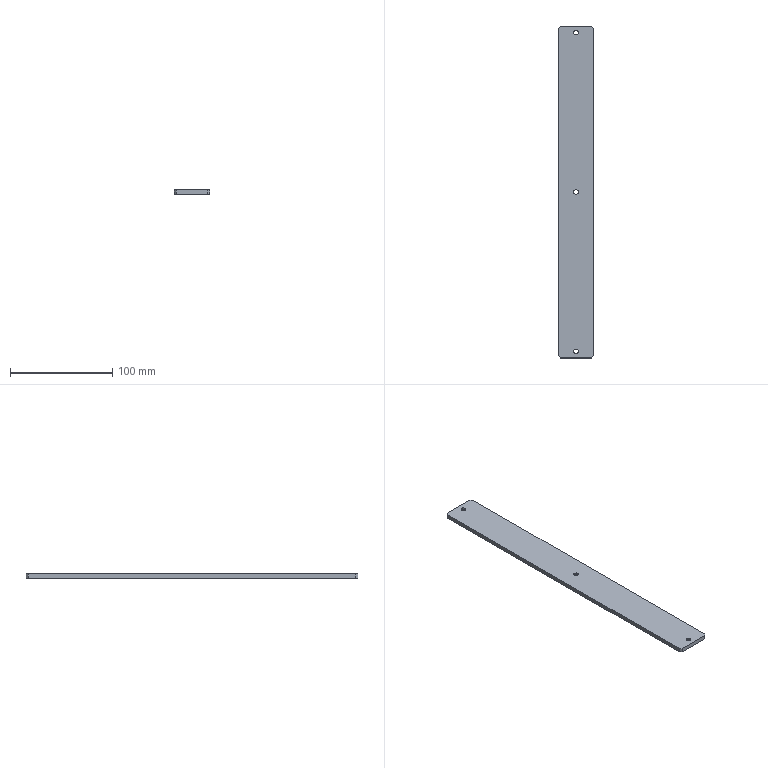Part | STEP file | 11-FG-SZ02811 | 1 solid | 22 faces | box 35 x 324 x 4 mm | volume 44997 mm3 | plane 10 | cone 6 | cylinder 6 | commonest cylinder face diameters 4.5 x6
STEP:
#1=CARTESIAN_POINT('',(2.25,-155.5,2.23));
#2=VERTEX_POINT('',#1);
#3=CARTESIAN_POINT('',(-2.25,-155.5,2.23));
#4=VERTEX_POINT('',#3);
#5=CARTESIAN_POINT('',(0.,-155.5,2.23));
#6=DIRECTION('',(0.,0.,-1.));
#7=DIRECTION('',(-1.,0.,0.));
#8=AXIS2_PLACEMENT_3D('',#5,#6,#7);
#9=CIRCLE('',#8,2.25);
#10=EDGE_CURVE('',#2,#4,#9,.T.);
#11=ORIENTED_EDGE('',*,*,#10,.F.);
#12=CARTESIAN_POINT('',(4.48,-155.5,0.));
#13=VERTEX_POINT('',#12);
#14=CARTESIAN_POINT('',(4.48,-155.5,0.));
#15=DIRECTION('',(0.7071,0.,-0.7071));
#16=VECTOR('',#15,1000.);
#17=LINE('',#14,#16);
#18=EDGE_CURVE('',#2,#13,#17,.T.);
#19=ORIENTED_EDGE('',*,*,#18,.T.);
#20=CARTESIAN_POINT('',(-4.48,-155.5,0.));
#21=VERTEX_POINT('',#20);
#22=CARTESIAN_POINT('',(0.,-155.5,0.));
#23=DIRECTION('',(0.,0.,-1.));
#24=DIRECTION('',(-1.,0.,0.));
#25=AXIS2_PLACEMENT_3D('',#22,#23,#24);
#26=CIRCLE('',#25,4.48);
#27=EDGE_CURVE('',#13,#21,#26,.T.);
#28=ORIENTED_EDGE('',*,*,#27,.T.);
#29=CARTESIAN_POINT('',(-4.48,-155.5,0.));
#30=DIRECTION('',(-0.7071,0.,-0.7071));
#31=VECTOR('',#30,1000.);
#32=LINE('',#29,#31);
#33=EDGE_CURVE('',#4,#21,#32,.T.);
#34=ORIENTED_EDGE('',*,*,#33,.F.);
#35=EDGE_LOOP('',(#11,#19,#28,#34));
#36=FACE_OUTER_BOUND('',#35,.T.);
#37=CARTESIAN_POINT('',(0.,-155.5,0.));
#38=DIRECTION('',(0.,0.,-1.));
#39=DIRECTION('',(-1.,0.,0.));
#40=AXIS2_PLACEMENT_3D('',#37,#38,#39);
#41=CONICAL_SURFACE('',#40,4.48,0.7854);
#42=ADVANCED_FACE('',(#36),#41,.F.);
#43=CARTESIAN_POINT('',(-2.25,-155.5,4.));
#44=VERTEX_POINT('',#43);
#45=CARTESIAN_POINT('',(2.25,-155.5,4.));
#46=VERTEX_POINT('',#45);
#47=CARTESIAN_POINT('',(0.,-155.5,4.));
#48=DIRECTION('',(0.,0.,1.));
#49=DIRECTION('',(1.,0.,0.));
#50=AXIS2_PLACEMENT_3D('',#47,#48,#49);
#51=CIRCLE('',#50,2.25);
#52=EDGE_CURVE('',#44,#46,#51,.T.);
#53=ORIENTED_EDGE('',*,*,#52,.T.);
#54=CARTESIAN_POINT('',(2.25,-155.5,0.));
#55=DIRECTION('',(0.,0.,-1.));
#56=VECTOR('',#55,1000.);
#57=LINE('',#54,#56);
#58=EDGE_CURVE('',#46,#2,#57,.T.);
#59=ORIENTED_EDGE('',*,*,#58,.T.);
#60=ORIENTED_EDGE('',*,*,#10,.T.);
#61=CARTESIAN_POINT('',(-2.25,-155.5,0.));
#62=DIRECTION('',(0.,0.,-1.));
#63=VECTOR('',#62,1000.);
#64=LINE('',#61,#63);
#65=EDGE_CURVE('',#44,#4,#64,.T.);
#66=ORIENTED_EDGE('',*,*,#65,.F.);
#67=EDGE_LOOP('',(#53,#59,#60,#66));
#68=FACE_OUTER_BOUND('',#67,.T.);
#69=CARTESIAN_POINT('',(0.,-155.5,0.));
#70=DIRECTION('',(0.,0.,-1.));
#71=DIRECTION('',(-1.,0.,0.));
#72=AXIS2_PLACEMENT_3D('',#69,#70,#71);
#73=CYLINDRICAL_SURFACE('',#72,2.25);
#74=ADVANCED_FACE('',(#68),#73,.F.);
#75=CARTESIAN_POINT('',(2.25,0.,2.23));
#76=VERTEX_POINT('',#75);
#77=CARTESIAN_POINT('',(-2.25,0.,2.23));
#78=VERTEX_POINT('',#77);
#79=CARTESIAN_POINT('',(0.,0.,2.23));
#80=DIRECTION('',(0.,0.,-1.));
#81=DIRECTION('',(-1.,0.,0.));
#82=AXIS2_PLACEMENT_3D('',#79,#80,#81);
#83=CIRCLE('',#82,2.25);
#84=EDGE_CURVE('',#76,#78,#83,.T.);
#85=ORIENTED_EDGE('',*,*,#84,.F.);
#86=CARTESIAN_POINT('',(4.48,0.,0.));
#87=VERTEX_POINT('',#86);
#88=CARTESIAN_POINT('',(4.48,0.,0.));
#89=DIRECTION('',(0.7071,0.,-0.7071));
#90=VECTOR('',#89,1000.);
#91=LINE('',#88,#90);
#92=EDGE_CURVE('',#76,#87,#91,.T.);
#93=ORIENTED_EDGE('',*,*,#92,.T.);
#94=CARTESIAN_POINT('',(-4.48,0.,0.));
#95=VERTEX_POINT('',#94);
#96=CARTESIAN_POINT('',(0.,0.,0.));
#97=DIRECTION('',(0.,0.,-1.));
#98=DIRECTION('',(-1.,0.,0.));
#99=AXIS2_PLACEMENT_3D('',#96,#97,#98);
#100=CIRCLE('',#99,4.48);
#101=EDGE_CURVE('',#87,#95,#100,.T.);
#102=ORIENTED_EDGE('',*,*,#101,.T.);
#103=CARTESIAN_POINT('',(-4.48,0.,0.));
#104=DIRECTION('',(-0.7071,0.,-0.7071));
#105=VECTOR('',#104,1000.);
#106=LINE('',#103,#105);
#107=EDGE_CURVE('',#78,#95,#106,.T.);
#108=ORIENTED_EDGE('',*,*,#107,.F.);
#109=EDGE_LOOP('',(#85,#93,#102,#108));
#110=FACE_OUTER_BOUND('',#109,.T.);
#111=CARTESIAN_POINT('',(0.,0.,0.));
#112=DIRECTION('',(0.,0.,-1.));
#113=DIRECTION('',(-1.,0.,0.));
#114=AXIS2_PLACEMENT_3D('',#111,#112,#113);
#115=CONICAL_SURFACE('',#114,4.48,0.7854);
#116=ADVANCED_FACE('',(#110),#115,.F.);
#117=CARTESIAN_POINT('',(-2.25,0.,4.));
#118=VERTEX_POINT('',#117);
#119=CARTESIAN_POINT('',(2.25,0.,4.));
#120=VERTEX_POINT('',#119);
#121=CARTESIAN_POINT('',(0.,0.,4.));
#122=DIRECTION('',(0.,0.,1.));
#123=DIRECTION('',(1.,0.,0.));
#124=AXIS2_PLACEMENT_3D('',#121,#122,#123);
#125=CIRCLE('',#124,2.25);
#126=EDGE_CURVE('',#118,#120,#125,.T.);
#127=ORIENTED_EDGE('',*,*,#126,.T.);
#128=CARTESIAN_POINT('',(2.25,0.,0.));
#129=DIRECTION('',(0.,0.,-1.));
#130=VECTOR('',#129,1000.);
#131=LINE('',#128,#130);
#132=EDGE_CURVE('',#120,#76,#131,.T.);
#133=ORIENTED_EDGE('',*,*,#132,.T.);
#134=ORIENTED_EDGE('',*,*,#84,.T.);
#135=CARTESIAN_POINT('',(-2.25,0.,0.));
#136=DIRECTION('',(0.,0.,-1.));
#137=VECTOR('',#136,1000.);
#138=LINE('',#135,#137);
#139=EDGE_CURVE('',#118,#78,#138,.T.);
#140=ORIENTED_EDGE('',*,*,#139,.F.);
#141=EDGE_LOOP('',(#127,#133,#134,#140));
#142=FACE_OUTER_BOUND('',#141,.T.);
#143=CARTESIAN_POINT('',(0.,0.,0.));
#144=DIRECTION('',(0.,0.,-1.));
#145=DIRECTION('',(-1.,0.,0.));
#146=AXIS2_PLACEMENT_3D('',#143,#144,#145);
#147=CYLINDRICAL_SURFACE('',#146,2.25);
#148=ADVANCED_FACE('',(#142),#147,.F.);
#149=CARTESIAN_POINT('',(2.25,155.5,2.23));
#150=VERTEX_POINT('',#149);
#151=CARTESIAN_POINT('',(-2.25,155.5,2.23));
#152=VERTEX_POINT('',#151);
#153=CARTESIAN_POINT('',(0.,155.5,2.23));
#154=DIRECTION('',(0.,0.,-1.));
#155=DIRECTION('',(-1.,0.,0.));
#156=AXIS2_PLACEMENT_3D('',#153,#154,#155);
#157=CIRCLE('',#156,2.25);
#158=EDGE_CURVE('',#150,#152,#157,.T.);
#159=ORIENTED_EDGE('',*,*,#158,.F.);
#160=CARTESIAN_POINT('',(4.48,155.5,0.));
#161=VERTEX_POINT('',#160);
#162=CARTESIAN_POINT('',(4.48,155.5,0.));
#163=DIRECTION('',(0.7071,0.,-0.7071));
#164=VECTOR('',#163,1000.);
#165=LINE('',#162,#164);
#166=EDGE_CURVE('',#150,#161,#165,.T.);
#167=ORIENTED_EDGE('',*,*,#166,.T.);
#168=CARTESIAN_POINT('',(-4.48,155.5,0.));
#169=VERTEX_POINT('',#168);
#170=CARTESIAN_POINT('',(0.,155.5,0.));
#171=DIRECTION('',(0.,0.,-1.));
#172=DIRECTION('',(-1.,0.,0.));
#173=AXIS2_PLACEMENT_3D('',#170,#171,#172);
#174=CIRCLE('',#173,4.48);
#175=EDGE_CURVE('',#161,#169,#174,.T.);
#176=ORIENTED_EDGE('',*,*,#175,.T.);
#177=CARTESIAN_POINT('',(-4.48,155.5,0.));
#178=DIRECTION('',(-0.7071,0.,-0.7071));
#179=VECTOR('',#178,1000.);
#180=LINE('',#177,#179);
#181=EDGE_CURVE('',#152,#169,#180,.T.);
#182=ORIENTED_EDGE('',*,*,#181,.F.);
#183=EDGE_LOOP('',(#159,#167,#176,#182));
#184=FACE_OUTER_BOUND('',#183,.T.);
#185=CARTESIAN_POINT('',(0.,155.5,0.));
#186=DIRECTION('',(0.,0.,-1.));
#187=DIRECTION('',(-1.,0.,0.));
#188=AXIS2_PLACEMENT_3D('',#185,#186,#187);
#189=CONICAL_SURFACE('',#188,4.48,0.7854);
#190=ADVANCED_FACE('',(#184),#189,.F.);
#191=CARTESIAN_POINT('',(-2.25,155.5,4.));
#192=VERTEX_POINT('',#191);
#193=CARTESIAN_POINT('',(2.25,155.5,4.));
#194=VERTEX_POINT('',#193);
#195=CARTESIAN_POINT('',(0.,155.5,4.));
#196=DIRECTION('',(0.,0.,1.));
#197=DIRECTION('',(1.,0.,0.));
#198=AXIS2_PLACEMENT_3D('',#195,#196,#197);
#199=CIRCLE('',#198,2.25);
#200=EDGE_CURVE('',#192,#194,#199,.T.);
#201=ORIENTED_EDGE('',*,*,#200,.T.);
#202=CARTESIAN_POINT('',(2.25,155.5,0.));
#203=DIRECTION('',(0.,0.,-1.));
#204=VECTOR('',#203,1000.);
#205=LINE('',#202,#204);
#206=EDGE_CURVE('',#194,#150,#205,.T.);
#207=ORIENTED_EDGE('',*,*,#206,.T.);
#208=ORIENTED_EDGE('',*,*,#158,.T.);
#209=CARTESIAN_POINT('',(-2.25,155.5,0.));
#210=DIRECTION('',(0.,0.,-1.));
#211=VECTOR('',#210,1000.);
#212=LINE('',#209,#211);
#213=EDGE_CURVE('',#192,#152,#212,.T.);
#214=ORIENTED_EDGE('',*,*,#213,.F.);
#215=EDGE_LOOP('',(#201,#207,#208,#214));
#216=FACE_OUTER_BOUND('',#215,.T.);
#217=CARTESIAN_POINT('',(0.,155.5,0.));
#218=DIRECTION('',(0.,0.,-1.));
#219=DIRECTION('',(-1.,0.,0.));
#220=AXIS2_PLACEMENT_3D('',#217,#218,#219);
#221=CYLINDRICAL_SURFACE('',#220,2.25);
#222=ADVANCED_FACE('',(#216),#221,.F.);
#223=CARTESIAN_POINT('',(-17.5,160.,0.));
#224=VERTEX_POINT('',#223);
#225=CARTESIAN_POINT('',(-17.5,-160.,0.));
#226=VERTEX_POINT('',#225);
#227=CARTESIAN_POINT('',(-17.5,-162.,0.));
#228=DIRECTION('',(0.,-1.,0.));
#229=VECTOR('',#228,1000.);
#230=LINE('',#227,#229);
#231=EDGE_CURVE('',#224,#226,#230,.T.);
#232=ORIENTED_EDGE('',*,*,#231,.T.);
#233=CARTESIAN_POINT('',(-17.5,-160.,4.));
#234=VERTEX_POINT('',#233);
#235=CARTESIAN_POINT('',(-17.5,-160.,4.));
#236=DIRECTION('',(0.,0.,1.));
#237=VECTOR('',#236,1000.);
#238=LINE('',#235,#237);
#239=EDGE_CURVE('',#226,#234,#238,.T.);
#240=ORIENTED_EDGE('',*,*,#239,.T.);
#241=CARTESIAN_POINT('',(-17.5,160.,4.));
#242=VERTEX_POINT('',#241);
#243=CARTESIAN_POINT('',(-17.5,-162.,4.));
#244=DIRECTION('',(0.,-1.,0.));
#245=VECTOR('',#244,1000.);
#246=LINE('',#243,#245);
#247=EDGE_CURVE('',#242,#234,#246,.T.);
#248=ORIENTED_EDGE('',*,*,#247,.F.);
#249=CARTESIAN_POINT('',(-17.5,160.,4.));
#250=DIRECTION('',(0.,0.,-1.));
#251=VECTOR('',#250,1000.);
#252=LINE('',#249,#251);
#253=EDGE_CURVE('',#242,#224,#252,.T.);
#254=ORIENTED_EDGE('',*,*,#253,.T.);
#255=EDGE_LOOP('',(#232,#240,#248,#254));
#256=FACE_OUTER_BOUND('',#255,.T.);
#257=CARTESIAN_POINT('',(-17.5,-162.,4.));
#258=DIRECTION('',(1.,0.,0.));
#259=DIRECTION('',(0.,0.,-1.));
#260=AXIS2_PLACEMENT_3D('',#257,#258,#259);
#261=PLANE('',#260);
#262=ADVANCED_FACE('',(#256),#261,.F.);
#263=CARTESIAN_POINT('',(-15.5,-162.,0.));
#264=VERTEX_POINT('',#263);
#265=CARTESIAN_POINT('',(15.5,-162.,0.));
#266=VERTEX_POINT('',#265);
#267=CARTESIAN_POINT('',(17.5,-162.,0.));
#268=DIRECTION('',(1.,0.,0.));
#269=VECTOR('',#268,1000.);
#270=LINE('',#267,#269);
#271=EDGE_CURVE('',#264,#266,#270,.T.);
#272=ORIENTED_EDGE('',*,*,#271,.T.);
#273=CARTESIAN_POINT('',(15.5,-162.,4.));
#274=VERTEX_POINT('',#273);
#275=CARTESIAN_POINT('',(15.5,-162.,4.));
#276=DIRECTION('',(0.,0.,1.));
#277=VECTOR('',#276,1000.);
#278=LINE('',#275,#277);
#279=EDGE_CURVE('',#266,#274,#278,.T.);
#280=ORIENTED_EDGE('',*,*,#279,.T.);
#281=CARTESIAN_POINT('',(-15.5,-162.,4.));
#282=VERTEX_POINT('',#281);
#283=CARTESIAN_POINT('',(17.5,-162.,4.));
#284=DIRECTION('',(1.,0.,0.));
#285=VECTOR('',#284,1000.);
#286=LINE('',#283,#285);
#287=EDGE_CURVE('',#282,#274,#286,.T.);
#288=ORIENTED_EDGE('',*,*,#287,.F.);
#289=CARTESIAN_POINT('',(-15.5,-162.,4.));
#290=DIRECTION('',(0.,0.,-1.));
#291=VECTOR('',#290,1000.);
#292=LINE('',#289,#291);
#293=EDGE_CURVE('',#282,#264,#292,.T.);
#294=ORIENTED_EDGE('',*,*,#293,.T.);
#295=EDGE_LOOP('',(#272,#280,#288,#294));
#296=FACE_OUTER_BOUND('',#295,.T.);
#297=CARTESIAN_POINT('',(17.5,-162.,4.));
#298=DIRECTION('',(0.,1.,0.));
#299=DIRECTION('',(0.,0.,1.));
#300=AXIS2_PLACEMENT_3D('',#297,#298,#299);
#301=PLANE('',#300);
#302=ADVANCED_FACE('',(#296),#301,.F.);
#303=CARTESIAN_POINT('',(17.5,-160.,4.));
#304=VERTEX_POINT('',#303);
#305=CARTESIAN_POINT('',(17.5,160.,4.));
#306=VERTEX_POINT('',#305);
#307=CARTESIAN_POINT('',(17.5,-162.,4.));
#308=DIRECTION('',(0.,1.,0.));
#309=VECTOR('',#308,1000.);
#310=LINE('',#307,#309);
#311=EDGE_CURVE('',#304,#306,#310,.T.);
#312=ORIENTED_EDGE('',*,*,#311,.F.);
#313=CARTESIAN_POINT('',(17.5,-160.,0.));
#314=VERTEX_POINT('',#313);
#315=CARTESIAN_POINT('',(17.5,-160.,4.));
#316=DIRECTION('',(0.,0.,-1.));
#317=VECTOR('',#316,1000.);
#318=LINE('',#315,#317);
#319=EDGE_CURVE('',#304,#314,#318,.T.);
#320=ORIENTED_EDGE('',*,*,#319,.T.);
#321=CARTESIAN_POINT('',(17.5,160.,0.));
#322=VERTEX_POINT('',#321);
#323=CARTESIAN_POINT('',(17.5,-162.,0.));
#324=DIRECTION('',(0.,1.,0.));
#325=VECTOR('',#324,1000.);
#326=LINE('',#323,#325);
#327=EDGE_CURVE('',#314,#322,#326,.T.);
#328=ORIENTED_EDGE('',*,*,#327,.T.);
#329=CARTESIAN_POINT('',(17.5,160.,4.));
#330=DIRECTION('',(0.,0.,1.));
#331=VECTOR('',#330,1000.);
#332=LINE('',#329,#331);
#333=EDGE_CURVE('',#322,#306,#332,.T.);
#334=ORIENTED_EDGE('',*,*,#333,.T.);
#335=EDGE_LOOP('',(#312,#320,#328,#334));
#336=FACE_OUTER_BOUND('',#335,.T.);
#337=CARTESIAN_POINT('',(17.5,-162.,4.));
#338=DIRECTION('',(-1.,0.,0.));
#339=DIRECTION('',(0.,0.,1.));
#340=AXIS2_PLACEMENT_3D('',#337,#338,#339);
#341=PLANE('',#340);
#342=ADVANCED_FACE('',(#336),#341,.F.);
#343=CARTESIAN_POINT('',(15.5,162.,4.));
#344=VERTEX_POINT('',#343);
#345=CARTESIAN_POINT('',(-15.5,162.,4.));
#346=VERTEX_POINT('',#345);
#347=CARTESIAN_POINT('',(17.5,162.,4.));
#348=DIRECTION('',(-1.,0.,0.));
#349=VECTOR('',#348,1000.);
#350=LINE('',#347,#349);
#351=EDGE_CURVE('',#344,#346,#350,.T.);
#352=ORIENTED_EDGE('',*,*,#351,.F.);
#353=CARTESIAN_POINT('',(15.5,162.,0.));
#354=VERTEX_POINT('',#353);
#355=CARTESIAN_POINT('',(15.5,162.,4.));
#356=DIRECTION('',(0.,0.,-1.));
#357=VECTOR('',#356,1000.);
#358=LINE('',#355,#357);
#359=EDGE_CURVE('',#344,#354,#358,.T.);
#360=ORIENTED_EDGE('',*,*,#359,.T.);
#361=CARTESIAN_POINT('',(-15.5,162.,0.));
#362=VERTEX_POINT('',#361);
#363=CARTESIAN_POINT('',(17.5,162.,0.));
#364=DIRECTION('',(-1.,0.,0.));
#365=VECTOR('',#364,1000.);
#366=LINE('',#363,#365);
#367=EDGE_CURVE('',#354,#362,#366,.T.);
#368=ORIENTED_EDGE('',*,*,#367,.T.);
#369=CARTESIAN_POINT('',(-15.5,162.,4.));
#370=DIRECTION('',(0.,0.,1.));
#371=VECTOR('',#370,1000.);
#372=LINE('',#369,#371);
#373=EDGE_CURVE('',#362,#346,#372,.T.);
#374=ORIENTED_EDGE('',*,*,#373,.T.);
#375=EDGE_LOOP('',(#352,#360,#368,#374));
#376=FACE_OUTER_BOUND('',#375,.T.);
#377=CARTESIAN_POINT('',(17.5,162.,4.));
#378=DIRECTION('',(0.,-1.,0.));
#379=DIRECTION('',(0.,0.,-1.));
#380=AXIS2_PLACEMENT_3D('',#377,#378,#379);
#381=PLANE('',#380);
#382=ADVANCED_FACE('',(#376),#381,.F.);
#383=ORIENTED_EDGE('',*,*,#52,.F.);
#384=CARTESIAN_POINT('',(0.,-155.5,4.));
#385=DIRECTION('',(0.,0.,1.));
#386=DIRECTION('',(1.,0.,0.));
#387=AXIS2_PLACEMENT_3D('',#384,#385,#386);
#388=CIRCLE('',#387,2.25);
#389=EDGE_CURVE('',#46,#44,#388,.T.);
#390=ORIENTED_EDGE('',*,*,#389,.F.);
#391=EDGE_LOOP('',(#383,#390));
#392=FACE_BOUND('',#391,.T.);
#393=ORIENTED_EDGE('',*,*,#126,.F.);
#394=CARTESIAN_POINT('',(0.,0.,4.));
#395=DIRECTION('',(0.,0.,1.));
#396=DIRECTION('',(1.,0.,0.));
#397=AXIS2_PLACEMENT_3D('',#394,#395,#396);
#398=CIRCLE('',#397,2.25);
#399=EDGE_CURVE('',#120,#118,#398,.T.);
#400=ORIENTED_EDGE('',*,*,#399,.F.);
#401=EDGE_LOOP('',(#393,#400));
#402=FACE_BOUND('',#401,.T.);
#403=ORIENTED_EDGE('',*,*,#200,.F.);
#404=CARTESIAN_POINT('',(0.,155.5,4.));
#405=DIRECTION('',(0.,0.,1.));
#406=DIRECTION('',(1.,0.,0.));
#407=AXIS2_PLACEMENT_3D('',#404,#405,#406);
#408=CIRCLE('',#407,2.25);
#409=EDGE_CURVE('',#194,#192,#408,.T.);
#410=ORIENTED_EDGE('',*,*,#409,.F.);
#411=EDGE_LOOP('',(#403,#410));
#412=FACE_BOUND('',#411,.T.);
#413=ORIENTED_EDGE('',*,*,#287,.T.);
#414=CARTESIAN_POINT('',(88.75,-88.75,4.));
#415=DIRECTION('',(0.7071,0.7071,0.));
#416=VECTOR('',#415,1000.);
#417=LINE('',#414,#416);
#418=EDGE_CURVE('',#274,#304,#417,.T.);
#419=ORIENTED_EDGE('',*,*,#418,.T.);
#420=ORIENTED_EDGE('',*,*,#311,.T.);
#421=CARTESIAN_POINT('',(88.75,88.75,4.));
#422=DIRECTION('',(-0.7071,0.7071,0.));
#423=VECTOR('',#422,1000.);
#424=LINE('',#421,#423);
#425=EDGE_CURVE('',#306,#344,#424,.T.);
#426=ORIENTED_EDGE('',*,*,#425,.T.);
#427=ORIENTED_EDGE('',*,*,#351,.T.);
#428=CARTESIAN_POINT('',(-88.75,88.75,4.));
#429=DIRECTION('',(-0.7071,-0.7071,0.));
#430=VECTOR('',#429,1000.);
#431=LINE('',#428,#430);
#432=EDGE_CURVE('',#346,#242,#431,.T.);
#433=ORIENTED_EDGE('',*,*,#432,.T.);
#434=ORIENTED_EDGE('',*,*,#247,.T.);
#435=CARTESIAN_POINT('',(-88.75,-88.75,4.));
#436=DIRECTION('',(0.7071,-0.7071,0.));
#437=VECTOR('',#436,1000.);
#438=LINE('',#435,#437);
#439=EDGE_CURVE('',#234,#282,#438,.T.);
#440=ORIENTED_EDGE('',*,*,#439,.T.);
#441=EDGE_LOOP('',(#413,#419,#420,#426,#427,#433,#434,#440));
#442=FACE_OUTER_BOUND('',#441,.T.);
#443=CARTESIAN_POINT('',(0.,0.,4.));
#444=DIRECTION('',(0.,0.,1.));
#445=DIRECTION('',(1.,0.,0.));
#446=AXIS2_PLACEMENT_3D('',#443,#444,#445);
#447=PLANE('',#446);
#448=ADVANCED_FACE('',(#392,#402,#412,#442),#447,.T.);
#449=CARTESIAN_POINT('',(0.,-155.5,0.));
#450=DIRECTION('',(0.,0.,-1.));
#451=DIRECTION('',(-1.,0.,0.));
#452=AXIS2_PLACEMENT_3D('',#449,#450,#451);
#453=CIRCLE('',#452,4.48);
#454=EDGE_CURVE('',#21,#13,#453,.T.);
#455=ORIENTED_EDGE('',*,*,#454,.F.);
#456=ORIENTED_EDGE('',*,*,#27,.F.);
#457=EDGE_LOOP('',(#455,#456));
#458=FACE_BOUND('',#457,.T.);
#459=CARTESIAN_POINT('',(0.,0.,0.));
#460=DIRECTION('',(0.,0.,-1.));
#461=DIRECTION('',(-1.,0.,0.));
#462=AXIS2_PLACEMENT_3D('',#459,#460,#461);
#463=CIRCLE('',#462,4.48);
#464=EDGE_CURVE('',#95,#87,#463,.T.);
#465=ORIENTED_EDGE('',*,*,#464,.F.);
#466=ORIENTED_EDGE('',*,*,#101,.F.);
#467=EDGE_LOOP('',(#465,#466));
#468=FACE_BOUND('',#467,.T.);
#469=CARTESIAN_POINT('',(0.,155.5,0.));
#470=DIRECTION('',(0.,0.,-1.));
#471=DIRECTION('',(-1.,0.,0.));
#472=AXIS2_PLACEMENT_3D('',#469,#470,#471);
#473=CIRCLE('',#472,4.48);
#474=EDGE_CURVE('',#169,#161,#473,.T.);
#475=ORIENTED_EDGE('',*,*,#474,.F.);
#476=ORIENTED_EDGE('',*,*,#175,.F.);
#477=EDGE_LOOP('',(#475,#476));
#478=FACE_BOUND('',#477,.T.);
#479=ORIENTED_EDGE('',*,*,#327,.F.);
#480=CARTESIAN_POINT('',(17.5,-160.,0.));
#481=DIRECTION('',(-0.7071,-0.7071,0.));
#482=VECTOR('',#481,1000.);
#483=LINE('',#480,#482);
#484=EDGE_CURVE('',#314,#266,#483,.T.);
#485=ORIENTED_EDGE('',*,*,#484,.T.);
#486=ORIENTED_EDGE('',*,*,#271,.F.);
#487=CARTESIAN_POINT('',(-15.5,-162.,0.));
#488=DIRECTION('',(-0.7071,0.7071,0.));
#489=VECTOR('',#488,1000.);
#490=LINE('',#487,#489);
#491=EDGE_CURVE('',#264,#226,#490,.T.);
#492=ORIENTED_EDGE('',*,*,#491,.T.);
#493=ORIENTED_EDGE('',*,*,#231,.F.);
#494=CARTESIAN_POINT('',(-17.5,160.,0.));
#495=DIRECTION('',(0.7071,0.7071,0.));
#496=VECTOR('',#495,1000.);
#497=LINE('',#494,#496);
#498=EDGE_CURVE('',#224,#362,#497,.T.);
#499=ORIENTED_EDGE('',*,*,#498,.T.);
#500=ORIENTED_EDGE('',*,*,#367,.F.);
#501=CARTESIAN_POINT('',(15.5,162.,0.));
#502=DIRECTION('',(0.7071,-0.7071,0.));
#503=VECTOR('',#502,1000.);
#504=LINE('',#501,#503);
#505=EDGE_CURVE('',#354,#322,#504,.T.);
#506=ORIENTED_EDGE('',*,*,#505,.T.);
#507=EDGE_LOOP('',(#479,#485,#486,#492,#493,#499,#500,#506));
#508=FACE_OUTER_BOUND('',#507,.T.);
#509=CARTESIAN_POINT('',(0.,0.,0.));
#510=DIRECTION('',(0.,0.,1.));
#511=DIRECTION('',(1.,0.,0.));
#512=AXIS2_PLACEMENT_3D('',#509,#510,#511);
#513=PLANE('',#512);
#514=ADVANCED_FACE('',(#458,#468,#478,#508),#513,.F.);
#515=ORIENTED_EDGE('',*,*,#206,.F.);
#516=ORIENTED_EDGE('',*,*,#409,.T.);
#517=ORIENTED_EDGE('',*,*,#213,.T.);
#518=CARTESIAN_POINT('',(0.,155.5,2.23));
#519=DIRECTION('',(0.,0.,-1.));
#520=DIRECTION('',(-1.,0.,0.));
#521=AXIS2_PLACEMENT_3D('',#518,#519,#520);
#522=CIRCLE('',#521,2.25);
#523=EDGE_CURVE('',#152,#150,#522,.T.);
#524=ORIENTED_EDGE('',*,*,#523,.T.);
#525=EDGE_LOOP('',(#515,#516,#517,#524));
#526=FACE_OUTER_BOUND('',#525,.T.);
#527=CARTESIAN_POINT('',(0.,155.5,0.));
#528=DIRECTION('',(0.,0.,-1.));
#529=DIRECTION('',(-1.,0.,0.));
#530=AXIS2_PLACEMENT_3D('',#527,#528,#529);
#531=CYLINDRICAL_SURFACE('',#530,2.25);
#532=ADVANCED_FACE('',(#526),#531,.F.);
#533=ORIENTED_EDGE('',*,*,#166,.F.);
#534=ORIENTED_EDGE('',*,*,#523,.F.);
#535=ORIENTED_EDGE('',*,*,#181,.T.);
#536=ORIENTED_EDGE('',*,*,#474,.T.);
#537=EDGE_LOOP('',(#533,#534,#535,#536));
#538=FACE_OUTER_BOUND('',#537,.T.);
#539=CARTESIAN_POINT('',(0.,155.5,0.));
#540=DIRECTION('',(0.,0.,-1.));
#541=DIRECTION('',(-1.,0.,0.));
#542=AXIS2_PLACEMENT_3D('',#539,#540,#541);
#543=CONICAL_SURFACE('',#542,4.48,0.7854);
#544=ADVANCED_FACE('',(#538),#543,.F.);
#545=ORIENTED_EDGE('',*,*,#132,.F.);
#546=ORIENTED_EDGE('',*,*,#399,.T.);
#547=ORIENTED_EDGE('',*,*,#139,.T.);
#548=CARTESIAN_POINT('',(0.,0.,2.23));
#549=DIRECTION('',(0.,0.,-1.));
#550=DIRECTION('',(-1.,0.,0.));
#551=AXIS2_PLACEMENT_3D('',#548,#549,#550);
#552=CIRCLE('',#551,2.25);
#553=EDGE_CURVE('',#78,#76,#552,.T.);
#554=ORIENTED_EDGE('',*,*,#553,.T.);
#555=EDGE_LOOP('',(#545,#546,#547,#554));
#556=FACE_OUTER_BOUND('',#555,.T.);
#557=CARTESIAN_POINT('',(0.,0.,0.));
#558=DIRECTION('',(0.,0.,-1.));
#559=DIRECTION('',(-1.,0.,0.));
#560=AXIS2_PLACEMENT_3D('',#557,#558,#559);
#561=CYLINDRICAL_SURFACE('',#560,2.25);
#562=ADVANCED_FACE('',(#556),#561,.F.);
#563=ORIENTED_EDGE('',*,*,#92,.F.);
#564=ORIENTED_EDGE('',*,*,#553,.F.);
#565=ORIENTED_EDGE('',*,*,#107,.T.);
#566=ORIENTED_EDGE('',*,*,#464,.T.);
#567=EDGE_LOOP('',(#563,#564,#565,#566));
#568=FACE_OUTER_BOUND('',#567,.T.);
#569=CARTESIAN_POINT('',(0.,0.,0.));
#570=DIRECTION('',(0.,0.,-1.));
#571=DIRECTION('',(-1.,0.,0.));
#572=AXIS2_PLACEMENT_3D('',#569,#570,#571);
#573=CONICAL_SURFACE('',#572,4.48,0.7854);
#574=ADVANCED_FACE('',(#568),#573,.F.);
#575=ORIENTED_EDGE('',*,*,#58,.F.);
#576=ORIENTED_EDGE('',*,*,#389,.T.);
#577=ORIENTED_EDGE('',*,*,#65,.T.);
#578=CARTESIAN_POINT('',(0.,-155.5,2.23));
#579=DIRECTION('',(0.,0.,-1.));
#580=DIRECTION('',(-1.,0.,0.));
#581=AXIS2_PLACEMENT_3D('',#578,#579,#580);
#582=CIRCLE('',#581,2.25);
#583=EDGE_CURVE('',#4,#2,#582,.T.);
#584=ORIENTED_EDGE('',*,*,#583,.T.);
#585=EDGE_LOOP('',(#575,#576,#577,#584));
#586=FACE_OUTER_BOUND('',#585,.T.);
#587=CARTESIAN_POINT('',(0.,-155.5,0.));
#588=DIRECTION('',(0.,0.,-1.));
#589=DIRECTION('',(-1.,0.,0.));
#590=AXIS2_PLACEMENT_3D('',#587,#588,#589);
#591=CYLINDRICAL_SURFACE('',#590,2.25);
#592=ADVANCED_FACE('',(#586),#591,.F.);
#593=ORIENTED_EDGE('',*,*,#18,.F.);
#594=ORIENTED_EDGE('',*,*,#583,.F.);
#595=ORIENTED_EDGE('',*,*,#33,.T.);
#596=ORIENTED_EDGE('',*,*,#454,.T.);
#597=EDGE_LOOP('',(#593,#594,#595,#596));
#598=FACE_OUTER_BOUND('',#597,.T.);
#599=CARTESIAN_POINT('',(0.,-155.5,0.));
#600=DIRECTION('',(0.,0.,-1.));
#601=DIRECTION('',(-1.,0.,0.));
#602=AXIS2_PLACEMENT_3D('',#599,#600,#601);
#603=CONICAL_SURFACE('',#602,4.48,0.7854);
#604=ADVANCED_FACE('',(#598),#603,.F.);
#605=ORIENTED_EDGE('',*,*,#418,.F.);
#606=ORIENTED_EDGE('',*,*,#279,.F.);
#607=ORIENTED_EDGE('',*,*,#484,.F.);
#608=ORIENTED_EDGE('',*,*,#319,.F.);
#609=EDGE_LOOP('',(#605,#606,#607,#608));
#610=FACE_OUTER_BOUND('',#609,.T.);
#611=CARTESIAN_POINT('',(17.5,-160.,4.));
#612=DIRECTION('',(-0.7071,0.7071,0.));
#613=DIRECTION('',(0.,0.,-1.));
#614=AXIS2_PLACEMENT_3D('',#611,#612,#613);
#615=PLANE('',#614);
#616=ADVANCED_FACE('',(#610),#615,.F.);
#617=ORIENTED_EDGE('',*,*,#439,.F.);
#618=ORIENTED_EDGE('',*,*,#239,.F.);
#619=ORIENTED_EDGE('',*,*,#491,.F.);
#620=ORIENTED_EDGE('',*,*,#293,.F.);
#621=EDGE_LOOP('',(#617,#618,#619,#620));
#622=FACE_OUTER_BOUND('',#621,.T.);
#623=CARTESIAN_POINT('',(-15.5,-162.,4.));
#624=DIRECTION('',(0.7071,0.7071,0.));
#625=DIRECTION('',(0.,0.,-1.));
#626=AXIS2_PLACEMENT_3D('',#623,#624,#625);
#627=PLANE('',#626);
#628=ADVANCED_FACE('',(#622),#627,.F.);
#629=ORIENTED_EDGE('',*,*,#425,.F.);
#630=ORIENTED_EDGE('',*,*,#333,.F.);
#631=ORIENTED_EDGE('',*,*,#505,.F.);
#632=ORIENTED_EDGE('',*,*,#359,.F.);
#633=EDGE_LOOP('',(#629,#630,#631,#632));
#634=FACE_OUTER_BOUND('',#633,.T.);
#635=CARTESIAN_POINT('',(15.5,162.,4.));
#636=DIRECTION('',(-0.7071,-0.7071,0.));
#637=DIRECTION('',(0.,0.,-1.));
#638=AXIS2_PLACEMENT_3D('',#635,#636,#637);
#639=PLANE('',#638);
#640=ADVANCED_FACE('',(#634),#639,.F.);
#641=ORIENTED_EDGE('',*,*,#432,.F.);
#642=ORIENTED_EDGE('',*,*,#373,.F.);
#643=ORIENTED_EDGE('',*,*,#498,.F.);
#644=ORIENTED_EDGE('',*,*,#253,.F.);
#645=EDGE_LOOP('',(#641,#642,#643,#644));
#646=FACE_OUTER_BOUND('',#645,.T.);
#647=CARTESIAN_POINT('',(-17.5,160.,4.));
#648=DIRECTION('',(0.7071,-0.7071,0.));
#649=DIRECTION('',(0.,0.,-1.));
#650=AXIS2_PLACEMENT_3D('',#647,#648,#649);
#651=PLANE('',#650);
#652=ADVANCED_FACE('',(#646),#651,.F.);
#653=CLOSED_SHELL('',(#42,#74,#116,#148,#190,#222,#262,#302,#342,#382,#448,#514,#532,#544,#562,#574,#592,#604,#616,#628,#640,#652));
#654=MANIFOLD_SOLID_BREP('',#653);
#655=CARTESIAN_POINT('',(0.,0.,0.));
#656=DIRECTION('',(0.,0.,1.));
#657=DIRECTION('',(1.,0.,0.));
#658=AXIS2_PLACEMENT_3D('',#655,#656,#657);
#659=(LENGTH_UNIT()NAMED_UNIT(*)SI_UNIT(.MILLI.,.METRE.));
#660=UNCERTAINTY_MEASURE_WITH_UNIT(LENGTH_MEASURE(0.00001),#659,'','');
#661=(NAMED_UNIT(*)PLANE_ANGLE_UNIT()SI_UNIT($,.RADIAN.));
#662=(NAMED_UNIT(*)SI_UNIT($,.STERADIAN.)SOLID_ANGLE_UNIT());
#663=(GEOMETRIC_REPRESENTATION_CONTEXT(3)GLOBAL_UNCERTAINTY_ASSIGNED_CONTEXT((#660))GLOBAL_UNIT_ASSIGNED_CONTEXT((#659,#661,#662))REPRESENTATION_CONTEXT('',''));
#664=ADVANCED_BREP_SHAPE_REPRESENTATION('',(#654,#658),#663);